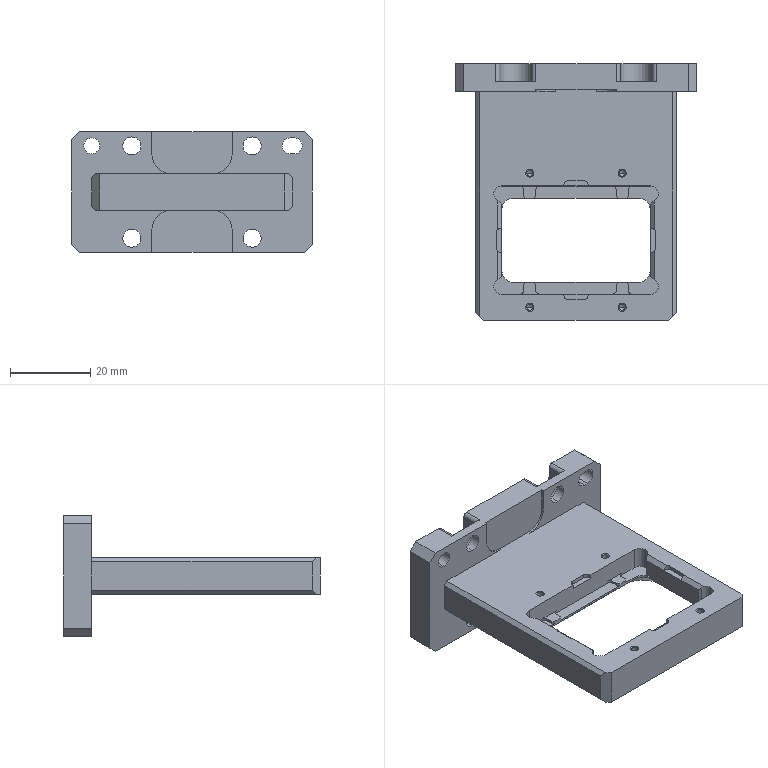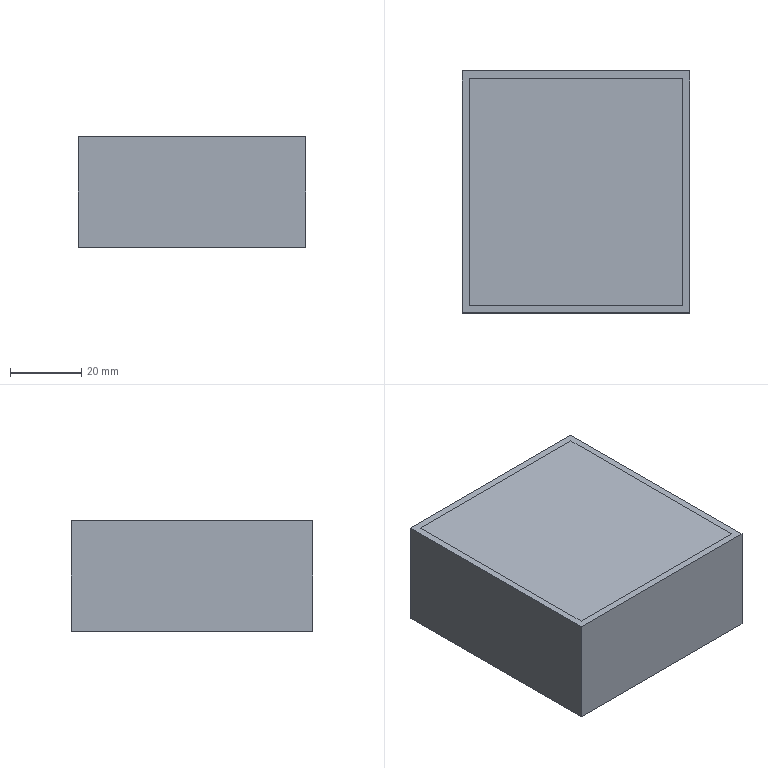CAM job | NX | 3+2 milling, drilling | part box 60 x 64 x 30 mm | stock box 64 x 68 x 31 mm
Operations:
program,operation,operation_type,tool,method,geometry_group,spindle_rpm,surface_speed,feed_per_tooth,feed_cut,feed_plunge,cut_length_mm,path_length_mm,cut_time_min,machine_time_min
1,FLOOR_WALL,VolumeBased25DMillingOperation,D20R0.8,METHOD,A,7500.0,471.0,0.09,1350.0,100.0,684.639,738.639,0.5071,0.5125
1,ZLEVEL_PROFILE,ZLevelMilling,D10,METHOD,A,9500.0,298.0,0.1579,3000.0,1000.0,41034.439,41122.389,13.693,13.702
1,ZLEVEL_PROFILE_COPY,ZLevelMilling,D10,METHOD,A,9500.0,298.0,0.0789,1500.0,1000.0,1891.842,1979.792,1.28,1.289
1,FLOOR_WALL_1,VolumeBased25DMillingOperation,D10,METHOD,A,9500.0,298.0,0.1579,3000.0,1000.0,38277.097,39853.835,12.887,13.045
1,FLOOR_WALL_1_COPY,VolumeBased25DMillingOperation,D10,METHOD,A,9500.0,298.0,0.0789,1500.0,1000.0,798.918,919.979,0.5351,0.5472
1,CAVITY_MILL,CavityMilling,D10,METHOD,A,9500.0,298.0,0.1579,3000.0,100.0,6993.563,8099.435,2.331,2.442
1,CAVITY_MILL_COPY,CavityMilling,D4,METHOD,A,9500.0,119.0,0.0947,1800.0,100.0,2594.898,7482.522,1.442,1.93
1,FLOOR_WALL_1_COPY_COPY,VolumeBased25DMillingOperation,D4,METHOD,A,9500.0,119.0,0.0789,1500.0,1000.0,556.535,2023.364,0.4058,0.5525
1,CAVITY_MILL_COPY_COPY,CavityMilling,D2,METHOD,A,9500.0,59.0,0.0632,1200.0,100.0,393.814,1153.481,0.3282,0.4041
1,ZLEVEL_PROFILE_COPY_1_COPY,ZLevelMilling,D4R0.5,METHOD,A,9500.0,119.0,0.1316,2500.0,100.0,890.89,959.59,0.3564,0.3632
1,DRILLING,Operation,D6A45,METHOD,A,5000.0,94.0,0.025,250.0,0.0,16.1,229.933,0.0644,0.0858
1,PLANAR_MILL_COPY,PlanarMilling,D6A45,METHOD,A,9500.0,179.0,0.0658,1250.0,500.0,203.976,393.576,0.1748,0.1938
1,PLANAR_MILL_COPY_COPY,PlanarMilling,D6A45,METHOD,A,9500.0,179.0,0.0658,1250.0,500.0,124.422,333.962,0.1112,0.1321
1,PLANAR_MILL_COPY_COPY_1,PlanarMilling,D6A45,METHOD,A,9500.0,179.0,0.0658,1250.0,500.0,133.328,257.9,0.1176,0.1301
1,PLANAR_MILL_COPY_COPY_1_COPY,PlanarMilling,D6A45,METHOD,A,9500.0,179.0,0.0658,1250.0,500.0,33.422,214.822,0.0384,0.0565
1,PLANAR_MILL_COPY_COPY_1_COPY_COPY,PlanarMilling,D6A45,METHOD,A,9500.0,179.0,0.0658,1250.0,500.0,58.494,248.094,0.0584,0.0774
1,刀补,ZLevelMilling,D4,METHOD,A,9500.0,298.0,0.0789,1500.0,1000.0,102.397,199.397,0.069,0.0787
1,ZLEVEL_PROFILE_COPY_COPY_COPY,ZLevelMilling,D4,METHOD,A,9500.0,298.0,0.0789,1500.0,1000.0,85.972,284.831,0.0595,0.0794
2,FLOOR_WALL_COPY,VolumeBased25DMillingOperation,D20R0.8,METHOD,B,7500.0,471.0,0.09,1350.0,100.0,652.639,706.639,0.4834,0.4888
2,FLOOR_WALL_1_COPY_1,VolumeBased25DMillingOperation,D10,METHOD,B,9500.0,298.0,0.1579,3000.0,1000.0,22082.939,23008.862,7.435,7.528
2,FLOOR_WALL_1_COPY_COPY_1,VolumeBased25DMillingOperation,D10,METHOD,B,9500.0,298.0,0.0789,1500.0,1000.0,798.918,919.979,0.5351,0.5472
2,ZLEVEL_PROFILE_COPY_1_COPY_COPY,ZLevelMilling,D4R0.5,METHOD,B,9500.0,119.0,0.1316,2500.0,100.0,890.449,959.149,0.3562,0.363
2,ZLEVEL_PROFILE_COPY_1_COPY_COPY_COPY_COPY,ZLevelMilling,D4R0.5,METHOD,B,9500.0,119.0,0.1316,2500.0,100.0,5392.947,5475.518,2.157,2.165
2,PLANAR_MILL_COPY_COPY_2,PlanarMilling,D6A45,METHOD,B,9500.0,179.0,0.0658,1250.0,500.0,55.711,132.211,0.0504,0.058
2,PLANAR_MILL_COPY_COPY_COPY,PlanarMilling,D6A45,METHOD,B,9500.0,179.0,0.0658,1250.0,500.0,124.422,333.962,0.1112,0.1321
2,PLANAR_MILL_COPY_COPY_1_COPY_1,PlanarMilling,D6A45,METHOD,B,9500.0,179.0,0.0658,1250.0,500.0,133.328,257.9,0.1176,0.1301
2,PLANAR_MILL_COPY_COPY_1_COPY_COPY_1,PlanarMilling,D6A45,METHOD,B,9500.0,179.0,0.0658,1250.0,500.0,33.422,214.822,0.0384,0.0565
3,ZLEVEL_PROFILE_1,ZLevelMilling,D6,METHOD,C,9500.0,179.0,0.0868,1650.0,100.0,970.613,1733.239,0.5883,0.6645
3,HOLE_MILLING,CylinderMilling,D3,METHOD,C,9500.0,89.0,0.0658,1250.0,100.0,210.856,593.058,0.1687,0.2069
3,HOLE_MILLING_COPY,CylinderMilling,D3,METHOD,C,9500.0,89.0,0.0658,1250.0,100.0,98.316,164.816,0.0787,0.0853
3,ZLEVEL_PROFILE_1_1,ZLevelMilling,D3,METHOD,C,9500.0,89.0,0.0632,1200.0,1000.0,184.312,249.312,0.1574,0.1639
3,PLANAR_MILL_COPY_COPY_1_COPY_2,PlanarMilling,D6A45,METHOD,C,9500.0,179.0,0.0658,1250.0,500.0,263.907,504.339,0.2257,0.2497
3,刀补3,CylinderMilling,D3,METHOD,C,9500.0,89.0,0.0658,1250.0,100.0,17.213,83.713,0.0138,0.0204
3,ZLEVEL_PROFILE_1_1_COPY,ZLevelMilling,D3,METHOD,C,9500.0,89.0,0.0632,1200.0,1000.0,27.274,94.024,0.023,0.0297